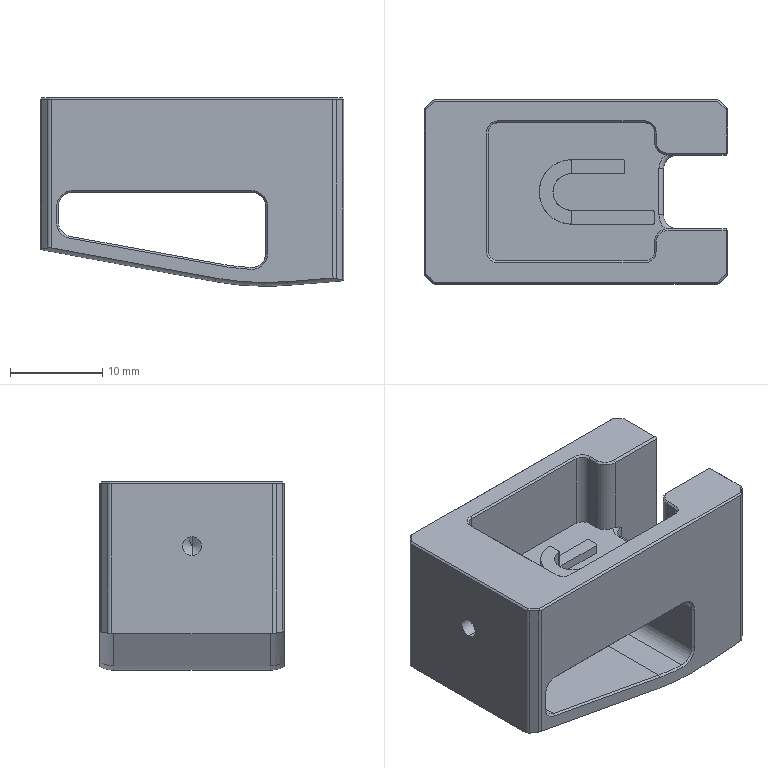NC program | NX | posted with a generic post | part box 33 x 20 x 20.478 mm
Lines 1477 to 3456 of 8500, first 1557 of 1976 lines:
(CAVITY_MILL_COPY , TOOL : D4)
N2934 T11 M6
N2936 G54
N2938 G17 G0 G90 X-6.7 Y-3.312 B0. C0. S9500 M3
N2940 G43 Z11. H11
N2942 Z1.21
N2944 G94 G1 Z-0.29 F1000.
N2946 X-7. Y-3.486
N2948 G3 X-7.5 Y-4.352 R1.
N2950 G1 Y-5.5 F1800.
N2952 X-6.352
N2954 G3 X-5.486 Y-5. R1.
N2956 G1 X-5.312 Y-4.7
N2958 Z1.21
N2960 G0 Z11.
N2962 X-6.7 Y-3.312
N2964 Z0.92
N2966 G1 Z-0.58 F1000.
N2968 X-7. Y-3.486
N2970 G3 X-7.5 Y-4.352 R1.
N2972 G1 Y-5.5 F1800.
N2974 X-6.352
N2976 G3 X-5.486 Y-5. R1.
N2978 G1 X-5.312 Y-4.7
N2980 Z0.92
N2982 G0 Z11.
N2984 X-6.7 Y-3.312
N2986 Z0.63
N2988 G1 Z-0.87 F1000.
N2990 X-7. Y-3.486
N2992 G3 X-7.5 Y-4.352 R1.
N2994 G1 Y-5.5 F1800.
N2996 X-6.352
N2998 G3 X-5.486 Y-5. R1.
N3000 G1 X-5.312 Y-4.7
N3002 Z0.63
N3004 G0 Z11.
N3006 X-6.7 Y-3.312
N3008 Z0.34
N3010 G1 Z-1.16 F1000.
N3012 X-7. Y-3.486
N3014 G3 X-7.5 Y-4.352 R1.
N3016 G1 Y-5.5 F1800.
N3018 X-6.352
N3020 G3 X-5.486 Y-5. R1.
N3022 G1 X-5.312 Y-4.7
N3024 Z0.34
N3026 G0 Z11.
N3028 X-6.7 Y-3.312
N3030 Z0.05
N3032 G1 Z-1.45 F1000.
N3034 X-7. Y-3.486
N3036 G3 X-7.5 Y-4.352 R1.
N3038 G1 Y-5.5 F1800.
N3040 X-6.352
N3042 G3 X-5.486 Y-5. R1.
N3044 G1 X-5.312 Y-4.7
N3046 Z0.05
N3048 G0 X-6.7 Y-3.312 Z-0.24
N3050 G1 Z-1.74 F1000.
N3052 X-7. Y-3.486
N3054 G3 X-7.5 Y-4.352 R1.
N3056 G1 Y-5.5 F1800.
N3058 X-6.352
N3060 G3 X-5.486 Y-5. R1.
N3062 G1 X-5.312 Y-4.7
N3064 Z-0.24
N3066 G0 X-6.7 Y-3.312 Z-0.53
N3068 G1 Z-2.03 F1000.
N3070 X-7. Y-3.486
N3072 G3 X-7.5 Y-4.352 R1.
N3074 G1 Y-5.5 F1800.
N3076 X-6.352
N3078 G3 X-5.486 Y-5. R1.
N3080 G1 X-5.312 Y-4.7
N3082 Z-0.53
N3084 G0 X-6.7 Y-3.312 Z-0.82
N3086 G1 Z-2.32 F1000.
N3088 X-7. Y-3.486
N3090 G3 X-7.5 Y-4.352 R1.
N3092 G1 Y-5.5 F1800.
N3094 X-6.352
N3096 G3 X-5.486 Y-5. R1.
N3098 G1 X-5.312 Y-4.7
N3100 Z-0.82
N3102 G0 X-6.7 Y-3.312 Z-1.11
N3104 G1 Z-2.61 F1000.
N3106 X-7. Y-3.486
N3108 G3 X-7.5 Y-4.352 R1.
N3110 G1 Y-5.5 F1800.
N3112 X-6.352
N3114 G3 X-5.486 Y-5. R1.
N3116 G1 X-5.312 Y-4.7
N3118 Z-1.11
N3120 G0 X-6.7 Y-3.312 Z-1.4
N3122 G1 Z-2.9 F1000.
N3124 X-7. Y-3.486
N3126 G3 X-7.5 Y-4.352 R1.
N3128 G1 Y-5.5 F1800.
N3130 X-6.352
N3132 G3 X-5.486 Y-5. R1.
N3134 G1 X-5.312 Y-4.7
N3136 Z-1.4
N3138 G0 X-6.7 Y-3.312 Z-1.69
N3140 G1 Z-3.19 F1000.
N3142 X-7. Y-3.486
N3144 G3 X-7.5 Y-4.352 R1.
N3146 G1 Y-5.5 F1800.
N3148 X-6.352
N3150 G3 X-5.486 Y-5. R1.
N3152 G1 X-5.312 Y-4.7
N3154 Z-1.69
N3156 G0 X-6.7 Y-3.312 Z-1.98
N3158 G1 Z-3.48 F1000.
N3160 X-7. Y-3.486
N3162 G3 X-7.5 Y-4.352 R1.
N3164 G1 Y-5.5 F1800.
N3166 X-6.352
N3168 G3 X-5.486 Y-5. R1.
N3170 G1 X-5.312 Y-4.7
N3172 Z-1.98
N3174 G0 X-6.7 Y-3.312 Z-2.27
N3176 G1 Z-3.77 F1000.
N3178 X-7. Y-3.486
N3180 G3 X-7.5 Y-4.352 R1.
N3182 G1 Y-5.5 F1800.
N3184 X-6.352
N3186 G3 X-5.486 Y-5. R1.
N3188 G1 X-5.312 Y-4.7
N3190 Z-2.27
N3192 G0 X-6.7 Y-3.312 Z-2.56
N3194 G1 Z-4.06 F1000.
N3196 X-7. Y-3.486
N3198 G3 X-7.5 Y-4.352 R1.
N3200 G1 Y-5.5 F1800.
N3202 X-6.352
N3204 G3 X-5.486 Y-5. R1.
N3206 G1 X-5.312 Y-4.7
N3208 Z-2.56
N3210 G0 X-6.7 Y-3.312 Z-2.85
N3212 G1 Z-4.35 F1000.
N3214 X-7. Y-3.486
N3216 G3 X-7.5 Y-4.352 R1.
N3218 G1 Y-5.5 F1800.
N3220 X-6.352
N3222 G3 X-5.486 Y-5. R1.
N3224 G1 X-5.312 Y-4.7
N3226 Z-2.85
N3228 G0 X-6.7 Y-3.312 Z-3.14
N3230 G1 Z-4.64 F1000.
N3232 X-7. Y-3.486
N3234 G3 X-7.5 Y-4.352 R1.
N3236 G1 Y-5.5 F1800.
N3238 X-6.352
N3240 G3 X-5.486 Y-5. R1.
N3242 G1 X-5.312 Y-4.7
N3244 Z-3.14
N3246 G0 X-6.7 Y-3.312 Z-3.43
N3248 G1 Z-4.93 F1000.
N3250 X-7. Y-3.486
N3252 G3 X-7.5 Y-4.352 R1.
N3254 G1 Y-5.5 F1800.
N3256 X-6.352
N3258 G3 X-5.486 Y-5. R1.
N3260 G1 X-5.312 Y-4.7
N3262 Z-3.43
N3264 G0 X-6.7 Y-3.312 Z-3.72
N3266 G1 Z-5.22 F1000.
N3268 X-7. Y-3.486
N3270 G3 X-7.5 Y-4.352 R1.
N3272 G1 Y-5.5 F1800.
N3274 X-6.352
N3276 G3 X-5.486 Y-5. R1.
N3278 G1 X-5.312 Y-4.7
N3280 Z-3.72
N3282 G0 X-6.7 Y-3.312 Z-4.01
N3284 G1 Z-5.51 F1000.
N3286 X-7. Y-3.486
N3288 G3 X-7.5 Y-4.352 R1.
N3290 G1 Y-5.5 F1800.
N3292 X-6.352
N3294 G3 X-5.486 Y-5. R1.
N3296 G1 X-5.312 Y-4.7
N3298 Z-4.01
N3300 G0 X-6.7 Y-3.312 Z-4.3
N3302 G1 Z-5.8 F1000.
N3304 X-7. Y-3.486
N3306 G3 X-7.5 Y-4.352 R1.
N3308 G1 Y-5.5 F1800.
N3310 X-6.352
N3312 G3 X-5.486 Y-5. R1.
N3314 G1 X-5.312 Y-4.7
N3316 Z-4.3
N3318 G0 X-6.7 Y-3.312 Z-4.586
N3320 G1 Z-6.086 F1000.
N3322 X-7. Y-3.486
N3324 G3 X-7.5 Y-4.352 R1.
N3326 G1 Y-5.5 F1800.
N3328 X-6.352
N3330 G3 X-5.486 Y-5. R1.
N3332 G1 X-5.845 Y-4.677
N3334 Z-4.586
N3336 G0 X-6.7 Y-3.312 Z-4.871
N3338 G1 Z-6.371 F1000.
N3340 X-7. Y-3.486
N3342 G3 X-7.5 Y-4.352 R1.
N3344 G1 Y-5.5 F1800.
N3346 X-6.352
N3348 G3 X-5.486 Y-5. R1.
N3350 G1 X-5.845 Y-4.677
N3352 Z-4.871
N3354 G0 X-6.7 Y-3.312 Z-5.157
N3356 G1 Z-6.657 F1000.
N3358 X-7. Y-3.486
N3360 G3 X-7.5 Y-4.352 R1.
N3362 G1 Y-5.5 F1800.
N3364 X-6.352
N3366 G3 X-5.486 Y-5. R1.
N3368 G1 X-5.845 Y-4.677
N3370 Z-5.157
N3372 G0 X-6.7 Y-3.312 Z-5.443
N3374 G1 Z-6.943 F1000.
N3376 X-7. Y-3.486
N3378 G3 X-7.5 Y-4.352 R1.
N3380 G1 Y-5.5 F1800.
N3382 X-6.352
N3384 G3 X-5.486 Y-5. R1.
N3386 G1 X-5.845 Y-4.677
N3388 Z-5.443
N3390 G0 X-6.7 Y-3.312 Z-5.729
N3392 G1 Z-7.229 F1000.
N3394 X-7. Y-3.486
N3396 G3 X-7.5 Y-4.352 R1.
N3398 G1 Y-5.5 F1800.
N3400 X-6.352
N3402 G3 X-5.486 Y-5. R1.
N3404 G1 X-5.845 Y-4.677
N3406 Z-5.729
N3408 G0 X-6.7 Y-3.312 Z-6.014
N3410 G1 Z-7.514 F1000.
N3412 X-7. Y-3.486
N3414 G3 X-7.5 Y-4.352 R1.
N3416 G1 Y-5.5 F1800.
N3418 X-6.352
N3420 G3 X-5.486 Y-5. R1.
N3422 G1 X-5.845 Y-4.677
N3424 Z-6.014
N3426 G0 X-6.7 Y-3.312 Z-6.3
N3428 G1 Z-7.8 F1000.
N3430 X-7. Y-3.486
N3432 G3 X-7.5 Y-4.352 R1.
N3434 G1 Y-5.5 F1800.
N3436 X-6.352
N3438 G3 X-5.486 Y-5. R1.
N3440 G1 X-5.845 Y-4.677
N3442 Z-6.3
N3444 G0 X-6.7 Y-3.312 Z-6.55
N3446 G1 Z-8.05 F1000.
N3448 X-7. Y-3.486
N3450 G3 X-7.5 Y-4.352 R1.
N3452 G1 Y-5.5 F1800.
N3454 X-6.352
N3456 G3 X-5.486 Y-5. R1.
N3458 G1 X-5.845 Y-4.677
N3460 Z-6.55
N3462 G0 X-6.7 Y-3.312 Z-6.8
N3464 G1 Z-8.3 F1000.
N3466 X-7. Y-3.486
N3468 G3 X-7.5 Y-4.352 R1.
N3470 G1 Y-5.5 F1800.
N3472 X-6.352
N3474 G3 X-5.486 Y-5. R1.
N3476 G1 X-5.845 Y-4.677
N3478 Z-6.8
N3480 G0 X-6.7 Y-3.312 Z-7.05
N3482 G1 Z-8.55 F1000.
N3484 X-7. Y-3.486
N3486 G3 X-7.5 Y-4.352 R1.
N3488 G1 Y-5.5 F1800.
N3490 X-6.352
N3492 G3 X-5.486 Y-5. R1.
N3494 G1 X-5.845 Y-4.677
N3496 Z-7.05
N3498 G0 X-6.7 Y-3.312 Z-7.3
N3500 G1 Z-8.8 F1000.
N3502 X-7. Y-3.486
N3504 G3 X-7.5 Y-4.352 R1.
N3506 G1 Y-5.5 F1800.
N3508 X-6.352
N3510 G3 X-5.486 Y-5. R1.
N3512 G1 X-5.845 Y-4.677
N3514 Z-7.3
N3516 G0 Z11.
N3518 X-5.518 Y-3.809
N3520 Z-4.586
N3522 G1 Z-6.086 F1000.
N3524 X-4.806 Y-3.721
N3526 G2 X-4.672 Y-4.712 R1.
N3528 X-5.005 Y-5.028 R0.56 F1800.
N3530 G3 X-5.339 Y-5.5 R0.5
N3532 G1 X2.412
N3534 G3 X2.078 Y-5.028 R0.5
N3536 G2 X1.707 Y-4.439 R0.56
N3538 G3 X1.407 Y-3.926 R0.5
N3540 G2 X-0.833 Y-5.49 R2.2
N3542 X-4.589 Y-3.678 R5.5
N3544 G3 X-4.687 Y-4.254 R0.5
N3546 G2 X-4.672 Y-4.712 R0.56
N3548 X-5.463 Y-5.324 R1.
N3550 G1 X-5.845 Y-4.677
N3552 Z-4.586
N3554 G0 X-5.518 Y-3.809 Z-4.871
N3556 G1 Z-6.371 F1000.
N3558 X-4.806 Y-3.721
N3560 G2 X-4.672 Y-4.712 R1.
N3562 X-5.005 Y-5.028 R0.56 F1800.
N3564 G3 X-5.339 Y-5.5 R0.5
N3566 G1 X2.412
N3568 G3 X2.078 Y-5.028 R0.5
N3570 G2 X1.707 Y-4.439 R0.56
N3572 G3 X1.407 Y-3.926 R0.5
N3574 G2 X-0.833 Y-5.49 R2.2
N3576 X-4.589 Y-3.678 R5.5
N3578 G3 X-4.687 Y-4.254 R0.5
N3580 G2 X-4.672 Y-4.712 R0.56
N3582 X-5.463 Y-5.324 R1.
N3584 G1 X-5.845 Y-4.677
N3586 Z-4.871
N3588 G0 X-5.518 Y-3.809 Z-5.157
N3590 G1 Z-6.657 F1000.
N3592 X-4.806 Y-3.721
N3594 G2 X-4.672 Y-4.712 R1.
N3596 X-5.005 Y-5.028 R0.56 F1800.
N3598 G3 X-5.339 Y-5.5 R0.5
N3600 G1 X2.412
N3602 G3 X2.078 Y-5.028 R0.5
N3604 G2 X1.707 Y-4.439 R0.56
N3606 G3 X1.407 Y-3.926 R0.5
N3608 G2 X-0.833 Y-5.49 R2.2
N3610 X-4.589 Y-3.678 R5.5
N3612 G3 X-4.687 Y-4.254 R0.5
N3614 G2 X-4.672 Y-4.712 R0.56
N3616 X-5.463 Y-5.324 R1.
N3618 G1 X-5.845 Y-4.677
N3620 Z-5.157
N3622 G0 X-5.518 Y-3.809 Z-5.443
N3624 G1 Z-6.943 F1000.
N3626 X-4.806 Y-3.721
N3628 G2 X-4.672 Y-4.712 R1.
N3630 X-5.005 Y-5.028 R0.56 F1800.
N3632 G3 X-5.339 Y-5.5 R0.5
N3634 G1 X2.412
N3636 G3 X2.078 Y-5.028 R0.5
N3638 G2 X1.707 Y-4.439 R0.56
N3640 G3 X1.407 Y-3.926 R0.5
N3642 G2 X-0.833 Y-5.49 R2.2
N3644 X-4.589 Y-3.678 R5.5
N3646 G3 X-4.687 Y-4.254 R0.5
N3648 G2 X-4.672 Y-4.712 R0.56
N3650 X-5.463 Y-5.324 R1.
N3652 G1 X-5.845 Y-4.677
N3654 Z-5.443
N3656 G0 X-5.518 Y-3.809 Z-5.729
N3658 G1 Z-7.229 F1000.
N3660 X-4.806 Y-3.721
N3662 G2 X-4.672 Y-4.712 R1.
N3664 X-5.005 Y-5.028 R0.56 F1800.
N3666 G3 X-5.339 Y-5.5 R0.5
N3668 G1 X2.412
N3670 G3 X2.078 Y-5.028 R0.5
N3672 G2 X1.707 Y-4.439 R0.56
N3674 G3 X1.407 Y-3.926 R0.5
N3676 G2 X-0.833 Y-5.49 R2.2
N3678 X-4.589 Y-3.678 R5.5
N3680 G3 X-4.687 Y-4.254 R0.5
N3682 G2 X-4.672 Y-4.712 R0.56
N3684 X-5.463 Y-5.324 R1.
N3686 G1 X-5.845 Y-4.677
N3688 Z-5.729
N3690 G0 X-5.518 Y-3.809 Z-6.014
N3692 G1 Z-7.514 F1000.
N3694 X-4.806 Y-3.721
N3696 G2 X-4.672 Y-4.712 R1.
N3698 X-5.005 Y-5.028 R0.56 F1800.
N3700 G3 X-5.339 Y-5.5 R0.5
N3702 G1 X2.412
N3704 G3 X2.078 Y-5.028 R0.5
N3706 G2 X1.707 Y-4.439 R0.56
N3708 G3 X1.407 Y-3.926 R0.5
N3710 G2 X-0.833 Y-5.49 R2.2
N3712 X-4.589 Y-3.678 R5.5
N3714 G3 X-4.687 Y-4.254 R0.5
N3716 G2 X-4.672 Y-4.712 R0.56
N3718 X-5.463 Y-5.324 R1.
N3720 G1 X-5.845 Y-4.677
N3722 Z-6.014
N3724 G0 X-5.518 Y-3.809 Z-6.3
N3726 G1 Z-7.8 F1000.
N3728 X-4.806 Y-3.721
N3730 G2 X-4.672 Y-4.712 R1.
N3732 X-5.005 Y-5.028 R0.56 F1800.
N3734 G3 X-5.339 Y-5.5 R0.5
N3736 G1 X2.412
N3738 G3 X2.078 Y-5.028 R0.5
N3740 G2 X1.707 Y-4.439 R0.56
N3742 G3 X1.407 Y-3.926 R0.5
N3744 G2 X-0.833 Y-5.49 R2.2
N3746 X-4.589 Y-3.678 R5.5
N3748 G3 X-4.687 Y-4.254 R0.5
N3750 G2 X-4.672 Y-4.712 R0.56
N3752 X-5.463 Y-5.324 R1.
N3754 G1 X-5.845 Y-4.677
N3756 Z-6.3
N3758 G0 Z-6.55
N3760 G1 Z-8.05 F1000.
N3762 X-6.205 Y-5.
N3764 G3 X-5.339 Y-5.5 R1.
N3766 G1 X-0.5 F1800.
N3768 G2 X-4.589 Y-3.678 R5.5
N3770 G3 X-5.54 Y-3.369 R1.
N3772 G1 X-5.79 Y-3.422
N3774 Z-6.55
N3776 G0 X-5.845 Y-4.677 Z-6.8
N3778 G1 Z-8.3 F1000.
N3780 X-6.205 Y-5.
N3782 G3 X-5.339 Y-5.5 R1.
N3784 G1 X-0.5 F1800.
N3786 G2 X-4.589 Y-3.678 R5.5
N3788 G3 X-5.54 Y-3.369 R1.
N3790 G1 X-5.79 Y-3.422
N3792 Z-6.8
N3794 G0 X-5.845 Y-4.677 Z-7.05
N3796 G1 Z-8.55 F1000.
N3798 X-6.205 Y-5.
N3800 G3 X-5.339 Y-5.5 R1.
N3802 G1 X-0.5 F1800.
N3804 G2 X-4.589 Y-3.678 R5.5
N3806 G3 X-5.54 Y-3.369 R1.
N3808 G1 X-5.79 Y-3.422
N3810 Z-7.05
N3812 G0 X-5.845 Y-4.677 Z-7.3
N3814 G1 Z-8.8 F1000.
N3816 X-6.205 Y-5.
N3818 G3 X-5.339 Y-5.5 R1.
N3820 G1 X-0.5 F1800.
N3822 G2 X-4.589 Y-3.678 R5.5
N3824 G3 X-5.54 Y-3.369 R1.
N3826 G1 X-5.79 Y-3.422
N3828 Z-7.3
N3830 G0 Z11.
N3832 X-5.312 Y4.7
N3834 Z1.21
N3836 G1 Z-0.29 F1000.
N3838 X-5.486 Y5.
N3840 G3 X-6.352 Y5.5 R1.
N3842 G1 X-7.5 F1800.
N3844 Y4.352
N3846 G3 X-7. Y3.486 R1.
N3848 G1 X-6.7 Y3.312
N3850 Z1.21
N3852 G0 Z11.
N3854 X-5.312 Y4.7
N3856 Z0.92
N3858 G1 Z-0.58 F1000.
N3860 X-5.486 Y5.
N3862 G3 X-6.352 Y5.5 R1.
N3864 G1 X-7.5 F1800.
N3866 Y4.352
N3868 G3 X-7. Y3.486 R1.
N3870 G1 X-6.7 Y3.312
N3872 Z0.92
N3874 G0 Z11.
N3876 X-5.312 Y4.7
N3878 Z0.63
N3880 G1 Z-0.87 F1000.
N3882 X-5.486 Y5.
N3884 G3 X-6.352 Y5.5 R1.
N3886 G1 X-7.5 F1800.
N3888 Y4.352
N3890 G3 X-7. Y3.486 R1.
N3892 G1 X-6.7 Y3.312
N3894 Z0.63
N3896 G0 Z11.
N3898 X-5.312 Y4.7
N3900 Z0.34
N3902 G1 Z-1.16 F1000.
N3904 X-5.486 Y5.
N3906 G3 X-6.352 Y5.5 R1.
N3908 G1 X-7.5 F1800.
N3910 Y4.352
N3912 G3 X-7. Y3.486 R1.
N3914 G1 X-6.7 Y3.312
N3916 Z0.34
N3918 G0 Z11.
N3920 X-5.312 Y4.7
N3922 Z0.05
N3924 G1 Z-1.45 F1000.
N3926 X-5.486 Y5.
N3928 G3 X-6.352 Y5.5 R1.
N3930 G1 X-7.5 F1800.
N3932 Y4.352
N3934 G3 X-7. Y3.486 R1.
N3936 G1 X-6.7 Y3.312
N3938 Z0.05
N3940 G0 X-5.312 Y4.7 Z-0.24
N3942 G1 Z-1.74 F1000.
N3944 X-5.486 Y5.
N3946 G3 X-6.352 Y5.5 R1.
N3948 G1 X-7.5 F1800.
N3950 Y4.352
N3952 G3 X-7. Y3.486 R1.
N3954 G1 X-6.7 Y3.312
N3956 Z-0.24
N3958 G0 X-5.312 Y4.7 Z-0.53
N3960 G1 Z-2.03 F1000.
N3962 X-5.486 Y5.
N3964 G3 X-6.352 Y5.5 R1.
N3966 G1 X-7.5 F1800.
N3968 Y4.352
N3970 G3 X-7. Y3.486 R1.
N3972 G1 X-6.7 Y3.312
N3974 Z-0.53
N3976 G0 X-5.312 Y4.7 Z-0.82
N3978 G1 Z-2.32 F1000.
N3980 X-5.486 Y5.
N3982 G3 X-6.352 Y5.5 R1.
N3984 G1 X-7.5 F1800.
N3986 Y4.352
N3988 G3 X-7. Y3.486 R1.
N3990 G1 X-6.7 Y3.312
N3992 Z-0.82
N3994 G0 X-5.312 Y4.7 Z-1.11
N3996 G1 Z-2.61 F1000.
N3998 X-5.486 Y5.
N4000 G3 X-6.352 Y5.5 R1.
N4002 G1 X-7.5 F1800.
N4004 Y4.352
N4006 G3 X-7. Y3.486 R1.
N4008 G1 X-6.7 Y3.312
N4010 Z-1.11
N4012 G0 X-5.312 Y4.7 Z-1.4
N4014 G1 Z-2.9 F1000.
N4016 X-5.486 Y5.
N4018 G3 X-6.352 Y5.5 R1.
N4020 G1 X-7.5 F1800.
N4022 Y4.352
N4024 G3 X-7. Y3.486 R1.
N4026 G1 X-6.7 Y3.312
N4028 Z-1.4
N4030 G0 X-5.312 Y4.7 Z-1.69
N4032 G1 Z-3.19 F1000.
N4034 X-5.486 Y5.
N4036 G3 X-6.352 Y5.5 R1.
N4038 G1 X-7.5 F1800.
N4040 Y4.352
N4042 G3 X-7. Y3.486 R1.
N4044 G1 X-6.7 Y3.312
N4046 Z-1.69
N4048 G0 X-5.312 Y4.7 Z-1.98
N4050 G1 Z-3.48 F1000.
N4052 X-5.486 Y5.
N4054 G3 X-6.352 Y5.5 R1.
N4056 G1 X-7.5 F1800.
N4058 Y4.352
N4060 G3 X-7. Y3.486 R1.
N4062 G1 X-6.7 Y3.312
N4064 Z-1.98
N4066 G0 X-5.312 Y4.7 Z-2.27
N4068 G1 Z-3.77 F1000.
N4070 X-5.486 Y5.
N4072 G3 X-6.352 Y5.5 R1.
N4074 G1 X-7.5 F1800.
N4076 Y4.352
N4078 G3 X-7. Y3.486 R1.
N4080 G1 X-6.7 Y3.312
N4082 Z-2.27
N4084 G0 X-5.312 Y4.7 Z-2.56
N4086 G1 Z-4.06 F1000.
N4088 X-5.486 Y5.
N4090 G3 X-6.352 Y5.5 R1.
N4092 G1 X-7.5 F1800.
N4094 Y4.352
N4096 G3 X-7. Y3.486 R1.
N4098 G1 X-6.7 Y3.312
N4100 Z-2.56
N4102 G0 X-5.312 Y4.7 Z-2.85
N4104 G1 Z-4.35 F1000.
N4106 X-5.486 Y5.
N4108 G3 X-6.352 Y5.5 R1.
N4110 G1 X-7.5 F1800.
N4112 Y4.352
N4114 G3 X-7. Y3.486 R1.
N4116 G1 X-6.7 Y3.312
N4118 Z-2.85
N4120 G0 X-5.312 Y4.7 Z-3.14
N4122 G1 Z-4.64 F1000.
N4124 X-5.486 Y5.
N4126 G3 X-6.352 Y5.5 R1.
N4128 G1 X-7.5 F1800.
N4130 Y4.352
N4132 G3 X-7. Y3.486 R1.
N4134 G1 X-6.7 Y3.312
N4136 Z-3.14
N4138 G0 X-5.312 Y4.7 Z-3.43
N4140 G1 Z-4.93 F1000.
N4142 X-5.486 Y5.
N4144 G3 X-6.352 Y5.5 R1.
N4146 G1 X-7.5 F1800.
N4148 Y4.352
N4150 G3 X-7. Y3.486 R1.
N4152 G1 X-6.7 Y3.312
N4154 Z-3.43
N4156 G0 X-5.312 Y4.7 Z-3.72
N4158 G1 Z-5.22 F1000.
N4160 X-5.486 Y5.
N4162 G3 X-6.352 Y5.5 R1.
N4164 G1 X-7.5 F1800.
N4166 Y4.352
N4168 G3 X-7. Y3.486 R1.
N4170 G1 X-6.7 Y3.312
N4172 Z-3.72
N4174 G0 X-5.312 Y4.7 Z-4.01
N4176 G1 Z-5.51 F1000.
N4178 X-5.486 Y5.
N4180 G3 X-6.352 Y5.5 R1.
N4182 G1 X-7.5 F1800.
N4184 Y4.352
N4186 G3 X-7. Y3.486 R1.
N4188 G1 X-6.7 Y3.312
N4190 Z-4.01
N4192 G0 X-5.312 Y4.7 Z-4.3
N4194 G1 Z-5.8 F1000.
N4196 X-5.486 Y5.
N4198 G3 X-6.352 Y5.5 R1.
N4200 G1 X-7.5 F1800.
N4202 Y4.352
N4204 G3 X-7. Y3.486 R1.
N4206 G1 X-6.7 Y3.312
N4208 Z-4.3
N4210 G0 X-6.429 Y-2.885 Z-4.586
N4212 G1 Z-6.086 F1000.
N4214 X-6.773 Y-2.576
N4216 G2 X-5.812 Y-2.299 R1.
N4218 G3 X-5.506 Y-2.277 R0.5 F1800.
N4220 G2 X-5.506 Y2.277 R5.5
N4222 G3 X-6.073 Y2.137 R0.5
N4224 G1 X-6.177 Y2.042
N4226 G3 X-6.5 Y1.771 R2.5
N4228 X-6.823 Y2.042 R2.5
N4230 G2 X-7.028 Y2.314 R0.56
N4232 G3 X-7.5 Y2.648 R0.5
N4234 G1 Y-2.648
N4236 G3 X-7.028 Y-2.314 R0.5
N4238 G2 X-6.823 Y-2.042 R0.56
N4240 G3 X-6.5 Y-1.771 R2.5
N4242 X-6.177 Y-2.042 R2.5
N4244 G1 X-6.073 Y-2.137
N4246 G3 X-5.812 Y-2.299 R0.5
N4248 G2 X-5.452 Y-2.645 R0.5
N4250 G1 X-5.997 Y-3.077
N4252 Z-4.586
N4254 G0 X-6.429 Y-2.885 Z-4.871
N4256 G1 Z-6.371 F1000.
N4258 X-6.773 Y-2.576
N4260 G2 X-5.812 Y-2.299 R1.
N4262 G3 X-5.506 Y-2.277 R0.5 F1800.
N4264 G2 X-5.506 Y2.277 R5.5
N4266 G3 X-6.073 Y2.137 R0.5
N4268 G1 X-6.177 Y2.042
N4270 G3 X-6.5 Y1.771 R2.5
N4272 X-6.823 Y2.042 R2.5
N4274 G2 X-7.028 Y2.314 R0.56
N4276 G3 X-7.5 Y2.648 R0.5
N4278 G1 Y-2.648
N4280 G3 X-7.028 Y-2.314 R0.5
N4282 G2 X-6.823 Y-2.042 R0.56
N4284 G3 X-6.5 Y-1.771 R2.5
N4286 X-6.177 Y-2.042 R2.5
N4288 G1 X-6.073 Y-2.137
N4290 G3 X-5.812 Y-2.299 R0.5
N4292 G2 X-5.452 Y-2.645 R0.5
N4294 G1 X-5.997 Y-3.077
N4296 Z-4.871
N4298 G0 X-6.429 Y-2.885 Z-5.157
N4300 G1 Z-6.657 F1000.
N4302 X-6.773 Y-2.576
N4304 G2 X-5.812 Y-2.299 R1.
N4306 G3 X-5.506 Y-2.277 R0.5 F1800.
N4308 G2 X-5.506 Y2.277 R5.5
N4310 G3 X-6.073 Y2.137 R0.5
N4312 G1 X-6.177 Y2.042
N4314 G3 X-6.5 Y1.771 R2.5
N4316 X-6.823 Y2.042 R2.5
N4318 G2 X-7.028 Y2.314 R0.56
N4320 G3 X-7.5 Y2.648 R0.5
N4322 G1 Y-2.648
N4324 G3 X-7.028 Y-2.314 R0.5
N4326 G2 X-6.823 Y-2.042 R0.56
N4328 G3 X-6.5 Y-1.771 R2.5
N4330 X-6.177 Y-2.042 R2.5
N4332 G1 X-6.073 Y-2.137
N4334 G3 X-5.812 Y-2.299 R0.5
N4336 G2 X-5.452 Y-2.645 R0.5
N4338 G1 X-5.997 Y-3.077
N4340 Z-5.157
N4342 G0 X-6.429 Y-2.885 Z-5.443
N4344 G1 Z-6.943 F1000.
N4346 X-6.773 Y-2.576
N4348 G2 X-5.812 Y-2.299 R1.
N4350 G3 X-5.506 Y-2.277 R0.5 F1800.
N4352 G2 X-5.506 Y2.277 R5.5
N4354 G3 X-6.073 Y2.137 R0.5
N4356 G1 X-6.177 Y2.042
N4358 G3 X-6.5 Y1.771 R2.5
N4360 X-6.823 Y2.042 R2.5
N4362 G2 X-7.028 Y2.314 R0.56
N4364 G3 X-7.5 Y2.648 R0.5
N4366 G1 Y-2.648
N4368 G3 X-7.028 Y-2.314 R0.5
N4370 G2 X-6.823 Y-2.042 R0.56
N4372 G3 X-6.5 Y-1.771 R2.5
N4374 X-6.177 Y-2.042 R2.5
N4376 G1 X-6.073 Y-2.137
N4378 G3 X-5.812 Y-2.299 R0.5
N4380 G2 X-5.452 Y-2.645 R0.5
N4382 G1 X-5.997 Y-3.077
N4384 Z-5.443
N4386 G0 X-6.429 Y-2.885 Z-5.729
N4388 G1 Z-7.229 F1000.
N4390 X-6.773 Y-2.576
N4392 G2 X-5.812 Y-2.299 R1.
N4394 G3 X-5.506 Y-2.277 R0.5 F1800.
N4396 G2 X-5.506 Y2.277 R5.5
N4398 G3 X-6.073 Y2.137 R0.5
N4400 G1 X-6.177 Y2.042
N4402 G3 X-6.5 Y1.771 R2.5
N4404 X-6.823 Y2.042 R2.5
N4406 G2 X-7.028 Y2.314 R0.56
N4408 G3 X-7.5 Y2.648 R0.5
N4410 G1 Y-2.648
N4412 G3 X-7.028 Y-2.314 R0.5
N4414 G2 X-6.823 Y-2.042 R0.56
N4416 G3 X-6.5 Y-1.771 R2.5
N4418 X-6.177 Y-2.042 R2.5
N4420 G1 X-6.073 Y-2.137
N4422 G3 X-5.812 Y-2.299 R0.5
N4424 G2 X-5.452 Y-2.645 R0.5
N4426 G1 X-5.997 Y-3.077
N4428 Z-5.729
N4430 G0 X-6.429 Y-2.885 Z-6.014
N4432 G1 Z-7.514 F1000.
N4434 X-6.773 Y-2.576
N4436 G2 X-5.812 Y-2.299 R1.
N4438 G3 X-5.506 Y-2.277 R0.5 F1800.
N4440 G2 X-5.506 Y2.277 R5.5
N4442 G3 X-6.073 Y2.137 R0.5
N4444 G1 X-6.177 Y2.042
N4446 G3 X-6.5 Y1.771 R2.5
N4448 X-6.823 Y2.042 R2.5
N4450 G2 X-7.028 Y2.314 R0.56
N4452 G3 X-7.5 Y2.648 R0.5
N4454 G1 Y-2.648
N4456 G3 X-7.028 Y-2.314 R0.5
N4458 G2 X-6.823 Y-2.042 R0.56
N4460 G3 X-6.5 Y-1.771 R2.5
N4462 X-6.177 Y-2.042 R2.5
N4464 G1 X-6.073 Y-2.137
N4466 G3 X-5.812 Y-2.299 R0.5
N4468 G2 X-5.452 Y-2.645 R0.5
N4470 G1 X-5.997 Y-3.077
N4472 Z-6.014
N4474 G0 X-6.429 Y-2.885 Z-6.3
N4476 G1 Z-7.8 F1000.
N4478 X-6.773 Y-2.576
N4480 G2 X-5.812 Y-2.299 R1.
N4482 G3 X-5.506 Y-2.277 R0.5 F1800.
N4484 G2 X-5.506 Y2.277 R5.5
N4486 G3 X-6.073 Y2.137 R0.5
N4488 G1 X-6.177 Y2.042
N4490 G3 X-6.5 Y1.771 R2.5
N4492 X-6.823 Y2.042 R2.5
N4494 G2 X-7.028 Y2.314 R0.56
N4496 G3 X-7.5 Y2.648 R0.5
N4498 G1 Y-2.648
N4500 G3 X-7.028 Y-2.314 R0.5
N4502 G2 X-6.823 Y-2.042 R0.56
N4504 G3 X-6.5 Y-1.771 R2.5
N4506 X-6.177 Y-2.042 R2.5
N4508 G1 X-6.073 Y-2.137
N4510 G3 X-5.812 Y-2.299 R0.5
N4512 G2 X-5.452 Y-2.645 R0.5
N4514 G1 X-5.997 Y-3.077
N4516 Z-6.3
N4518 G0 X-6.429 Y-2.885 Z-6.55
N4520 G1 Z-8.05 F1000.
N4522 X-6.773 Y-2.576
N4524 G2 X-5.812 Y-2.299 R1.
N4526 G3 X-5.506 Y-2.277 R0.5 F1800.
N4528 G2 X-5.506 Y2.277 R5.5
N4530 G3 X-6.073 Y2.137 R0.5
N4532 G1 X-6.177 Y2.042
N4534 G3 X-6.5 Y1.771 R2.5
N4536 X-6.823 Y2.042 R2.5
N4538 G2 X-7.028 Y2.314 R0.56
N4540 G3 X-7.5 Y2.648 R0.5
N4542 G1 Y-2.648
N4544 G3 X-7.028 Y-2.314 R0.5
N4546 G2 X-6.823 Y-2.042 R0.56
N4548 G3 X-6.5 Y-1.771 R2.5
N4550 X-6.177 Y-2.042 R2.5
N4552 G1 X-6.073 Y-2.137
N4554 G3 X-5.812 Y-2.299 R0.5
N4556 G2 X-5.452 Y-2.645 R0.5
N4558 G1 X-5.997 Y-3.077
N4560 Z-6.55
N4562 G0 X-6.429 Y-2.885 Z-6.8
N4564 G1 Z-8.3 F1000.
N4566 X-6.773 Y-2.576
N4568 G2 X-5.812 Y-2.299 R1.
N4570 G3 X-5.506 Y-2.277 R0.5 F1800.
N4572 G2 X-5.506 Y2.277 R5.5
N4574 G3 X-6.073 Y2.137 R0.5
N4576 G1 X-6.177 Y2.042
N4578 G3 X-6.5 Y1.771 R2.5
N4580 X-6.823 Y2.042 R2.5
N4582 G2 X-7.028 Y2.314 R0.56
N4584 G3 X-7.5 Y2.648 R0.5
N4586 G1 Y-2.648
N4588 G3 X-7.028 Y-2.314 R0.5
N4590 G2 X-6.823 Y-2.042 R0.56
N4592 G3 X-6.5 Y-1.771 R2.5
N4594 X-6.177 Y-2.042 R2.5
N4596 G1 X-6.073 Y-2.137
N4598 G3 X-5.812 Y-2.299 R0.5
N4600 G2 X-5.452 Y-2.645 R0.5
N4602 G1 X-5.997 Y-3.077
N4604 Z-6.8
N4606 G0 X-6.429 Y-2.885 Z-7.05
N4608 G1 Z-8.55 F1000.
N4610 X-6.773 Y-2.576
N4612 G2 X-5.812 Y-2.299 R1.
N4614 G3 X-5.506 Y-2.277 R0.5 F1800.
N4616 G2 X-5.506 Y2.277 R5.5
N4618 G3 X-6.073 Y2.137 R0.5
N4620 G1 X-6.177 Y2.042
N4622 G3 X-6.5 Y1.771 R2.5
N4624 X-6.823 Y2.042 R2.5
N4626 G2 X-7.028 Y2.314 R0.56
N4628 G3 X-7.5 Y2.648 R0.5
N4630 G1 Y-2.648
N4632 G3 X-7.028 Y-2.314 R0.5
N4634 G2 X-6.823 Y-2.042 R0.56
N4636 G3 X-6.5 Y-1.771 R2.5
N4638 X-6.177 Y-2.042 R2.5
N4640 G1 X-6.073 Y-2.137
N4642 G3 X-5.812 Y-2.299 R0.5
N4644 G2 X-5.452 Y-2.645 R0.5
N4646 G1 X-5.997 Y-3.077
N4648 Z-7.05
N4650 G0 X-6.429 Y-2.885 Z-7.3
N4652 G1 Z-8.8 F1000.
N4654 X-6.773 Y-2.576
N4656 G2 X-5.812 Y-2.299 R1.
N4658 G3 X-5.506 Y-2.277 R0.5 F1800.
N4660 G2 X-5.506 Y2.277 R5.5
N4662 G3 X-6.073 Y2.137 R0.5
N4664 G1 X-6.177 Y2.042
N4666 G3 X-6.5 Y1.771 R2.5
N4668 X-6.823 Y2.042 R2.5
N4670 G2 X-7.028 Y2.314 R0.56
N4672 G3 X-7.5 Y2.648 R0.5
N4674 G1 Y-2.648
N4676 G3 X-7.028 Y-2.314 R0.5
N4678 G2 X-6.823 Y-2.042 R0.56
N4680 G3 X-6.5 Y-1.771 R2.5
N4682 X-6.177 Y-2.042 R2.5
N4684 G1 X-6.073 Y-2.137
N4686 G3 X-5.812 Y-2.299 R0.5
N4688 G2 X-5.452 Y-2.645 R0.5
N4690 G1 X-5.997 Y-3.077
N4692 Z-7.3
N4694 G0 Z11.
N4696 X-5.864 Y4.655
N4698 Z-4.586
N4700 G1 Z-6.086 F1000.
N4702 X-5.486 Y5.
N4704 G3 X-6.352 Y5.5 R1.
N4706 G1 X-7.5 F1800.
N4708 Y4.352
N4710 G3 X-7. Y3.486 R1.
N4712 G1 X-6.7 Y3.312
N4714 Z-4.586
N4716 G0 X-5.864 Y4.655 Z-4.871
N4718 G1 Z-6.371 F1000.
N4720 X-5.486 Y5.
N4722 G3 X-6.352 Y5.5 R1.
N4724 G1 X-7.5 F1800.
N4726 Y4.352
N4728 G3 X-7. Y3.486 R1.
N4730 G1 X-6.7 Y3.312
N4732 Z-4.871
N4734 G0 X-5.864 Y4.655 Z-5.157
N4736 G1 Z-6.657 F1000.
N4738 X-5.486 Y5.
N4740 G3 X-6.352 Y5.5 R1.
N4742 G1 X-7.5 F1800.
N4744 Y4.352
N4746 G3 X-7. Y3.486 R1.
N4748 G1 X-6.7 Y3.312
N4750 Z-5.157
N4752 G0 X-5.864 Y4.655 Z-5.443
N4754 G1 Z-6.943 F1000.
N4756 X-5.486 Y5.
N4758 G3 X-6.352 Y5.5 R1.
N4760 G1 X-7.5 F1800.
N4762 Y4.352
N4764 G3 X-7. Y3.486 R1.
N4766 G1 X-6.7 Y3.312
N4768 Z-5.443
N4770 G0 X-5.864 Y4.655 Z-5.729
N4772 G1 Z-7.229 F1000.
N4774 X-5.486 Y5.
N4776 G3 X-6.352 Y5.5 R1.
N4778 G1 X-7.5 F1800.
N4780 Y4.352
N4782 G3 X-7. Y3.486 R1.
N4784 G1 X-6.7 Y3.312
N4786 Z-5.729
N4788 G0 X-5.864 Y4.655 Z-6.014
N4790 G1 Z-7.514 F1000.
N4792 X-5.486 Y5.
N4794 G3 X-6.352 Y5.5 R1.
N4796 G1 X-7.5 F1800.
N4798 Y4.352
N4800 G3 X-7. Y3.486 R1.
N4802 G1 X-6.7 Y3.312
N4804 Z-6.014
N4806 G0 X-5.864 Y4.655 Z-6.3
N4808 G1 Z-7.8 F1000.
N4810 X-5.486 Y5.
N4812 G3 X-6.352 Y5.5 R1.
N4814 G1 X-7.5 F1800.
N4816 Y4.352
N4818 G3 X-7. Y3.486 R1.
N4820 G1 X-6.7 Y3.312
N4822 Z-6.3
N4824 G0 X-5.864 Y4.655 Z-6.55
N4826 G1 Z-8.05 F1000.
N4828 X-5.486 Y5.
N4830 G3 X-6.352 Y5.5 R1.
N4832 G1 X-7.5 F1800.
N4834 Y4.352
N4836 G3 X-7. Y3.486 R1.
N4838 G1 X-6.7 Y3.312
N4840 Z-6.55
N4842 G0 X-5.864 Y4.655 Z-6.8
N4844 G1 Z-8.3 F1000.
N4846 X-5.486 Y5.
N4848 G3 X-6.352 Y5.5 R1.
N4850 G1 X-7.5 F1800.
N4852 Y4.352
N4854 G3 X-7. Y3.486 R1.
N4856 G1 X-6.7 Y3.312
N4858 Z-6.8
N4860 G0 X-5.864 Y4.655 Z-7.05
N4862 G1 Z-8.55 F1000.
N4864 X-5.486 Y5.
N4866 G3 X-6.352 Y5.5 R1.
N4868 G1 X-7.5 F1800.
N4870 Y4.352
N4872 G3 X-7. Y3.486 R1.
N4874 G1 X-6.7 Y3.312
N4876 Z-7.05
N4878 G0 X-5.864 Y4.655 Z-7.3
N4880 G1 Z-8.8 F1000.
N4882 X-5.486 Y5.
N4884 G3 X-6.352 Y5.5 R1.
N4886 G1 X-7.5 F1800.
N4888 Y4.352
N4890 G3 X-7. Y3.486 R1.
N4892 G1 X-6.7 Y3.312
N4894 Z-7.3
N4896 G0 Z11.
N4898 X-5.864 Y4.655
N4900 Z-4.586
N4902 G1 Z-6.086 F1000.
N4904 X-5.469 Y5.334
N4906 G2 X-4.702 Y4.692 R1.
N4908 X-4.745 Y4.216 R0.56 F1800.
N4910 G3 X-4.658 Y3.6 R0.5
N4912 G2 X-0.833 Y5.49 R5.5
N4914 X1.407 Y3.926 R2.2
N4916 G3 X1.707 Y4.439 R0.5
N4918 G2 X2.078 Y5.028 R0.56
N4920 G3 X2.412 Y5.5 R0.5
N4922 G1 X-5.376
N4924 G3 X-5.042 Y5.028 R0.5
N4926 G2 X-4.702 Y4.692 R0.56
N4928 X-4.874 Y3.707 R1.
N4930 G1 X-5.589 Y3.713
N4932 Z-4.586
N4934 G0 X-5.864 Y4.655 Z-4.871
N4936 G1 Z-6.371 F1000.
N4938 X-5.469 Y5.334
N4940 G2 X-4.702 Y4.692 R1.
N4942 X-4.745 Y4.216 R0.56 F1800.
N4944 G3 X-4.658 Y3.6 R0.5
N4946 G2 X-0.833 Y5.49 R5.5
N4948 X1.407 Y3.926 R2.2
N4950 G3 X1.707 Y4.439 R0.5
N4952 G2 X2.078 Y5.028 R0.56
N4954 G3 X2.412 Y5.5 R0.5
N4956 G1 X-5.376
N4958 G3 X-5.042 Y5.028 R0.5
N4960 G2 X-4.702 Y4.692 R0.56
N4962 X-4.874 Y3.707 R1.
N4964 G1 X-5.589 Y3.713
N4966 Z-4.871
N4968 G0 X-5.864 Y4.655 Z-5.157
N4970 G1 Z-6.657 F1000.
N4972 X-5.469 Y5.334
N4974 G2 X-4.702 Y4.692 R1.
N4976 X-4.745 Y4.216 R0.56 F1800.
N4978 G3 X-4.658 Y3.6 R0.5
N4980 G2 X-0.833 Y5.49 R5.5
N4982 X1.407 Y3.926 R2.2
N4984 G3 X1.707 Y4.439 R0.5
N4986 G2 X2.078 Y5.028 R0.56
N4988 G3 X2.412 Y5.5 R0.5
N4990 G1 X-5.376
N4992 G3 X-5.042 Y5.028 R0.5
N4994 G2 X-4.702 Y4.692 R0.56
N4996 X-4.874 Y3.707 R1.
N4998 G1 X-5.589 Y3.713
N5000 Z-5.157
N5002 G0 X-5.864 Y4.655 Z-5.443
N5004 G1 Z-6.943 F1000.
N5006 X-5.469 Y5.334
N5008 G2 X-4.702 Y4.692 R1.
N5010 X-4.745 Y4.216 R0.56 F1800.
N5012 G3 X-4.658 Y3.6 R0.5
N5014 G2 X-0.833 Y5.49 R5.5
N5016 X1.407 Y3.926 R2.2
N5018 G3 X1.707 Y4.439 R0.5
N5020 G2 X2.078 Y5.028 R0.56
N5022 G3 X2.412 Y5.5 R0.5
N5024 G1 X-5.376
N5026 G3 X-5.042 Y5.028 R0.5
N5028 G2 X-4.702 Y4.692 R0.56
N5030 X-4.874 Y3.707 R1.
N5032 G1 X-5.589 Y3.713
N5034 Z-5.443
N5036 G0 X-5.864 Y4.655 Z-5.729
N5038 G1 Z-7.229 F1000.
N5040 X-5.469 Y5.334
N5042 G2 X-4.702 Y4.692 R1.
N5044 X-4.745 Y4.216 R0.56 F1800.
N5046 G3 X-4.658 Y3.6 R0.5
N5048 G2 X-0.833 Y5.49 R5.5
N5050 X1.407 Y3.926 R2.2
N5052 G3 X1.707 Y4.439 R0.5
N5054 G2 X2.078 Y5.028 R0.56
N5056 G3 X2.412 Y5.5 R0.5
N5058 G1 X-5.376
N5060 G3 X-5.042 Y5.028 R0.5
N5062 G2 X-4.702 Y4.692 R0.56
N5064 X-4.874 Y3.707 R1.
N5066 G1 X-5.589 Y3.713
N5068 Z-5.729
N5070 G0 X-5.864 Y4.655 Z-6.014
N5072 G1 Z-7.514 F1000.
N5074 X-5.469 Y5.334
N5076 G2 X-4.702 Y4.692 R1.
N5078 X-4.745 Y4.216 R0.56 F1800.
N5080 G3 X-4.658 Y3.6 R0.5
N5082 G2 X-0.833 Y5.49 R5.5
N5084 X1.407 Y3.926 R2.2
N5086 G3 X1.707 Y4.439 R0.5
N5088 G2 X2.078 Y5.028 R0.56
N5090 G3 X2.412 Y5.5 R0.5
N5092 G1 X-5.376
N5094 G3 X-5.042 Y5.028 R0.5
N5096 G2 X-4.702 Y4.692 R0.56
N5098 X-4.874 Y3.707 R1.
N5100 G1 X-5.589 Y3.713
N5102 Z-6.014
N5104 G0 X-5.864 Y4.655 Z-6.3
N5106 G1 Z-7.8 F1000.
N5108 X-5.469 Y5.334
N5110 G2 X-4.702 Y4.692 R1.
N5112 X-4.745 Y4.216 R0.56 F1800.
N5114 G3 X-4.658 Y3.6 R0.5
N5116 G2 X-0.833 Y5.49 R5.5
N5118 X1.407 Y3.926 R2.2
N5120 G3 X1.707 Y4.439 R0.5
N5122 G2 X2.078 Y5.028 R0.56
N5124 G3 X2.412 Y5.5 R0.5
N5126 G1 X-5.376
N5128 G3 X-5.042 Y5.028 R0.5
N5130 G2 X-4.702 Y4.692 R0.56
N5132 X-4.874 Y3.707 R1.
N5134 G1 X-5.589 Y3.713
N5136 Z-6.3
N5138 G0 X-5.852 Y3.323 Z-6.55
N5140 G1 Z-8.05 F1000.
N5142 X-5.602 Y3.275
N5144 G3 X-4.657 Y3.602 R1.
N5146 G2 X-0.678 Y5.5 R5.503 F1800.
N5148 G1 X-5.376
N5150 G3 X-6.242 Y5. R1.
N5152 G1 X-5.864 Y4.655
N5154 Z-6.55
N5156 G0 X-5.852 Y3.323 Z-6.8
N5158 G1 Z-8.3 F1000.
N5160 X-5.602 Y3.275
N5162 G3 X-4.657 Y3.602 R1.
N5164 G2 X-0.678 Y5.5 R5.503 F1800.
N5166 G1 X-5.376
N5168 G3 X-6.242 Y5. R1.
N5170 G1 X-5.864 Y4.655
N5172 Z-6.8
N5174 G0 X-5.852 Y3.323 Z-7.05
N5176 G1 Z-8.55 F1000.
N5178 X-5.602 Y3.275
N5180 G3 X-4.657 Y3.602 R1.
N5182 G2 X-0.678 Y5.5 R5.503 F1800.
N5184 G1 X-5.376
N5186 G3 X-6.242 Y5. R1.
N5188 G1 X-5.864 Y4.655
N5190 Z-7.05
N5192 G0 X-5.852 Y3.323 Z-7.3
N5194 G1 Z-8.8 F1000.
N5196 X-5.602 Y3.275
N5198 G3 X-4.657 Y3.602 R1.
N5200 G2 X-0.678 Y5.5 R5.503 F1800.
N5202 G1 X-5.376
N5204 G3 X-6.242 Y5. R1.
N5206 G1 X-5.864 Y4.655
N5208 Z-7.3
N5210 G0 Z11.
N5212 X2.132 Y1.2
N5214 Z-4.586
N5216 G1 Z-6.086 F1000.
N5218 X1.965 Y1.222
N5220 G3 X1.039 Y0.844 R1.
N5222 G2 X-0.5 Y0. R2.2 F1800.
N5224 X1.039 Y-0.844 R2.2
N5226 G3 X1.965 Y-1.222 R1.
N5228 G1 X2.132 Y-1.2
N5230 Z-4.586
N5232 G0 Y1.2 Z-4.871
N5234 G1 Z-6.371 F1000.
N5236 X1.965 Y1.222
N5238 G3 X1.039 Y0.844 R1.
N5240 G2 X-0.5 Y0. R2.2 F1800.
N5242 X1.039 Y-0.844 R2.2
N5244 G3 X1.965 Y-1.222 R1.
N5246 G1 X2.132 Y-1.2
N5248 Z-4.871
N5250 G0 Y1.2 Z-5.157
N5252 G1 Z-6.657 F1000.
N5254 X1.965 Y1.222
N5256 G3 X1.039 Y0.844 R1.
N5258 G2 X-0.5 Y0. R2.2 F1800.
N5260 X1.039 Y-0.844 R2.2
N5262 G3 X1.965 Y-1.222 R1.
N5264 G1 X2.132 Y-1.2
N5266 Z-5.157
N5268 G0 Y1.2 Z-5.443
N5270 G1 Z-6.943 F1000.
N5272 X1.965 Y1.222
N5274 G3 X1.039 Y0.844 R1.
N5276 G2 X-0.5 Y0. R2.2 F1800.
N5278 X1.039 Y-0.844 R2.2
N5280 G3 X1.965 Y-1.222 R1.
N5282 G1 X2.132 Y-1.2
N5284 Z-5.443
N5286 G0 Y1.2 Z-5.729
N5288 G1 Z-7.229 F1000.
N5290 X1.965 Y1.222
N5292 G3 X1.039 Y0.844 R1.
N5294 G2 X-0.5 Y0. R2.2 F1800.
N5296 X1.039 Y-0.844 R2.2
N5298 G3 X1.965 Y-1.222 R1.
N5300 G1 X2.132 Y-1.2
N5302 Z-5.729
N5304 G0 Y1.2 Z-6.014
N5306 G1 Z-7.514 F1000.
N5308 X1.965 Y1.222
N5310 G3 X1.039 Y0.844 R1.
N5312 G2 X-0.5 Y0. R2.2 F1800.
N5314 X1.039 Y-0.844 R2.2
N5316 G3 X1.965 Y-1.222 R1.
N5318 G1 X2.132 Y-1.2
N5320 Z-6.014
N5322 G0 Y1.2 Z-6.3
N5324 G1 Z-7.8 F1000.
N5326 X1.965 Y1.222
N5328 G3 X1.039 Y0.844 R1.
N5330 G2 X-0.5 Y0. R2.2 F1800.
N5332 X1.039 Y-0.844 R2.2
N5334 G3 X1.965 Y-1.222 R1.
N5336 G1 X2.132 Y-1.2
N5338 Z-6.3
N5340 G0 Z11.
N5342 X6.241 Y3.412
N5344 Z1.21
N5346 G1 Z-0.29 F1000.
N5348 X6.392 Y3.568
N5350 G3 X6.635 Y4.538 R1.
N5352 G2 X6.5 Y5.5 R3.5 F1800.
N5354 G1 X5.464
N5356 G3 X4.598 Y5. R1.
N5358 G1 X4.425 Y4.7
N5360 Z1.21
N5362 G0 Z11.
N5364 X6.241 Y3.411
N5366 Z0.92
N5368 G1 Z-0.58 F1000.
N5370 X6.392 Y3.567
N5372 G3 X6.635 Y4.538 R1.
N5374 G2 X6.5 Y5.5 R3.5 F1800.
N5376 G1 X5.464
N5378 G3 X4.598 Y5. R1.
N5380 G1 X4.425 Y4.7
N5382 Z0.92
N5384 G0 Z11.
N5386 X6.242 Y3.411
N5388 Z0.63
N5390 G1 Z-0.87 F1000.
N5392 X6.393 Y3.567
N5394 G3 X6.635 Y4.537 R1.
N5396 G2 X6.5 Y5.5 R3.5 F1800.
N5398 G1 X5.464
N5400 G3 X4.598 Y5. R1.
N5402 G1 X4.425 Y4.7
N5404 Z0.63
N5406 G0 Z11.
N5408 X6.242 Y3.411
N5410 Z0.34
N5412 G1 Z-1.16 F1000.
N5414 X6.393 Y3.567
N5416 G3 X6.635 Y4.537 R1.
N5418 G2 X6.5 Y5.5 R3.5 F1800.
N5420 G1 X5.464
N5422 G3 X4.598 Y5. R1.
N5424 G1 X4.424 Y4.7
N5426 Z0.34
N5428 G0 Z11.
N5430 X6.242 Y3.41
N5432 Z0.05
N5434 G1 Z-1.45 F1000.
N5436 X6.393 Y3.566
N5438 G3 X6.635 Y4.537 R1.
N5440 G2 X6.5 Y5.5 R3.5 F1800.
N5442 G1 X5.463
N5444 G3 X4.597 Y5. R1.
N5446 G1 X4.424 Y4.7
N5448 Z0.05
N5450 G0 X6.242 Y3.41 Z-0.24
N5452 G1 Z-1.74 F1000.
N5454 X6.393 Y3.566
N5456 G3 X6.635 Y4.536 R1.
N5458 G2 X6.5 Y5.5 R3.5 F1800.
N5460 G1 X5.463
N5462 G3 X4.597 Y5. R1.
N5464 G1 X4.424 Y4.7
N5466 Z-0.24
N5468 G0 X6.242 Y3.41 Z-0.53
N5470 G1 Z-2.03 F1000.
N5472 X6.393 Y3.566
N5474 G3 X6.635 Y4.536 R1.
N5476 G2 X6.5 Y5.5 R3.5 F1800.
N5478 G1 X5.463
N5480 G3 X4.597 Y5. R1.
N5482 G1 X4.424 Y4.7
N5484 Z-0.53
N5486 G0 X6.243 Y3.409 Z-0.82
N5488 G1 Z-2.32 F1000.
N5490 X6.393 Y3.565
N5492 G3 X6.635 Y4.536 R1.
N5494 G2 X6.5 Y5.5 R3.5 F1800.
N5496 G1 X5.463
N5498 G3 X4.597 Y5. R1.
N5500 G1 X4.424 Y4.7
N5502 Z-0.82
N5504 G0 X6.243 Y3.409 Z-1.11
N5506 G1 Z-2.61 F1000.
N5508 X6.394 Y3.565
N5510 G3 X6.636 Y4.535 R1.
N5512 G2 X6.5 Y5.5 R3.5 F1800.
N5514 G1 X5.463
N5516 G3 X4.597 Y5. R1.
N5518 G1 X4.424 Y4.7
N5520 Z-1.11
N5522 G0 X6.243 Y3.408 Z-1.4
N5524 G1 Z-2.9 F1000.
N5526 X6.394 Y3.565
N5528 G3 X6.636 Y4.535 R1.
N5530 G2 X6.5 Y5.5 R3.5 F1800.
N5532 G1 X5.463
N5534 G3 X4.597 Y5. R1.
N5536 G1 X4.424 Y4.7
N5538 Z-1.4
N5540 G0 X6.243 Y3.408 Z-1.69
N5542 G1 Z-3.19 F1000.
N5544 X6.394 Y3.564
N5546 G3 X6.636 Y4.535 R1.
N5548 G2 X6.5 Y5.5 R3.5 F1800.
N5550 G1 X5.463
N5552 G3 X4.597 Y5. R1.
N5554 G1 X4.423 Y4.7
N5556 Z-1.69
N5558 G0 X6.243 Y3.408 Z-1.98
N5560 G1 Z-3.48 F1000.
N5562 X6.394 Y3.564
N5564 G3 X6.636 Y4.534 R1.
N5566 G2 X6.5 Y5.5 R3.5 F1800.
N5568 G1 X5.462
N5570 G3 X4.596 Y5. R1.
N5572 G1 X4.423 Y4.7
N5574 Z-1.98
N5576 G0 X6.244 Y3.407 Z-2.27
N5578 G1 Z-3.77 F1000.
N5580 X6.394 Y3.564
N5582 G3 X6.636 Y4.534 R1.
N5584 G2 X6.5 Y5.5 R3.5 F1800.
N5586 G1 X5.462
N5588 G3 X4.596 Y5. R1.
N5590 G1 X4.423 Y4.7
N5592 Z-2.27
N5594 G0 X6.244 Y3.407 Z-2.56
N5596 G1 Z-4.06 F1000.
N5598 X6.395 Y3.563
N5600 G3 X6.636 Y4.534 R1.
N5602 G2 X6.5 Y5.5 R3.5 F1800.
N5604 G1 X5.462
N5606 G3 X4.596 Y5. R1.
N5608 G1 X4.423 Y4.7
N5610 Z-2.56
N5612 G0 X6.244 Y3.407 Z-2.85
N5614 G1 Z-4.35 F1000.
N5616 X6.395 Y3.563
N5618 G3 X6.636 Y4.533 R1.
N5620 G2 X6.5 Y5.5 R3.5 F1800.
N5622 G1 X5.462
N5624 G3 X4.596 Y5. R1.
N5626 G1 X4.423 Y4.7
N5628 Z-2.85
N5630 G0 X6.244 Y3.406 Z-3.14
N5632 G1 Z-4.64 F1000.
N5634 X6.395 Y3.563
N5636 G3 X6.636 Y4.533 R1.
N5638 G2 X6.5 Y5.5 R3.5 F1800.
N5640 G1 X5.462
N5642 G3 X4.596 Y5. R1.
N5644 G1 X4.423 Y4.7
N5646 Z-3.14
N5648 G0 X6.244 Y3.406 Z-3.43
N5650 G1 Z-4.93 F1000.
N5652 X6.395 Y3.562
N5654 G3 X6.636 Y4.533 R1.
N5656 G2 X6.5 Y5.5 R3.5 F1800.
N5658 G1 X5.462
N5660 G3 X4.596 Y5. R1.
N5662 G1 X4.423 Y4.7
N5664 Z-3.43
N5666 G0 X6.245 Y3.406 Z-3.72
N5668 G1 Z-5.22 F1000.
N5670 X6.395 Y3.562
N5672 G3 X6.636 Y4.533 R1.
N5674 G2 X6.5 Y5.5 R3.5 F1800.
N5676 G1 X5.462
N5678 G3 X4.596 Y5. R1.
N5680 G1 X4.422 Y4.7
N5682 Z-3.72
N5684 G0 X6.245 Y3.405 Z-4.01
N5686 G1 Z-5.51 F1000.
N5688 X6.395 Y3.562
N5690 G3 X6.636 Y4.532 R1.
N5692 G2 X6.5 Y5.5 R3.5 F1800.
N5694 G1 X5.462
N5696 G3 X4.595 Y5. R1.
N5698 G1 X4.422 Y4.7
N5700 Z-4.01
N5702 G0 X6.245 Y3.405 Z-4.3
N5704 G1 Z-5.8 F1000.
N5706 X6.396 Y3.561
N5708 G3 X6.637 Y4.532 R1.
N5710 G2 X6.5 Y5.5 R3.5 F1800.
N5712 G1 X5.461
N5714 G3 X4.595 Y5. R1.
N5716 G1 X4.422 Y4.7
N5718 Z-4.3
N5720 G0 X6.245 Y3.405 Z-4.586
N5722 G1 Z-6.086 F1000.
N5724 X6.396 Y3.561
N5726 G3 X6.637 Y4.532 R1.
N5728 G2 X6.5 Y5.5 R3.5 F1800.
N5730 G1 X5.461
N5732 G3 X4.595 Y5. R1.
N5734 G1 X4.422 Y4.7
N5736 Z-4.586
N5738 G0 X6.245 Y3.404 Z-4.871
N5740 G1 Z-6.371 F1000.
N5742 X6.396 Y3.561
N5744 G3 X6.637 Y4.531 R1.
N5746 G2 X6.5 Y5.5 R3.5 F1800.
N5748 G1 X5.461
N5750 G3 X4.595 Y5. R1.
N5752 G1 X4.422 Y4.7
N5754 Z-4.871
N5756 G0 X6.245 Y3.404 Z-5.157
N5758 G1 Z-6.657 F1000.
N5760 X6.396 Y3.56
N5762 G3 X6.637 Y4.531 R1.
N5764 G2 X6.5 Y5.5 R3.5 F1800.
N5766 G1 X5.461
N5768 G3 X4.595 Y5. R1.
N5770 G1 X4.422 Y4.7
N5772 Z-5.157
N5774 G0 X6.246 Y3.404 Z-5.443
N5776 G1 Z-6.943 F1000.
N5778 X6.396 Y3.56
N5780 G3 X6.637 Y4.531 R1.
N5782 G2 X6.5 Y5.5 R3.5 F1800.
N5784 G1 X5.461
N5786 G3 X4.595 Y5. R1.
N5788 G1 X4.422 Y4.7
N5790 Z-5.443
N5792 G0 X6.246 Y3.403 Z-5.729
N5794 G1 Z-7.229 F1000.
N5796 X6.397 Y3.56
N5798 G3 X6.637 Y4.53 R1.
N5800 G2 X6.5 Y5.5 R3.5 F1800.
N5802 G1 X5.461
N5804 G3 X4.595 Y5. R1.
N5806 G1 X4.421 Y4.7
N5808 Z-5.729
N5810 G0 X6.246 Y3.403 Z-6.014
N5812 G1 Z-7.514 F1000.
N5814 X6.397 Y3.559
N5816 G3 X6.637 Y4.53 R1.
N5818 G2 X6.5 Y5.5 R3.5 F1800.
N5820 G1 X5.461
N5822 G3 X4.595 Y5. R1.
N5824 G1 X4.421 Y4.7
N5826 Z-6.014
N5828 G0 X6.246 Y3.403 Z-6.3
N5830 G1 Z-7.8 F1000.
N5832 X6.397 Y3.559
N5834 G3 X6.637 Y4.53 R1.
N5836 G2 X6.5 Y5.5 R3.5 F1800.
N5838 G1 X5.46
N5840 G3 X4.594 Y5. R1.
N5842 G1 X4.421 Y4.7
N5844 Z-6.3
N5846 G0 X9.442 Y1.236 Z-6.55
N5848 G1 Z-8.05 F1000.
N5850 X9.406 Y1.451
N5852 G3 X8.771 Y2.223 R1.
N5854 G2 X7.3 Y3.273 R3.5 F1800.
N5856 G1 Y2.2
N5858 G2 X5.1 Y0. R2.2
N5860 G1 X8.215
N5862 G3 X9.081 Y0.5 R1.
N5864 G1 X9.179 Y0.668
N5866 Z-6.55
N5868 G0 X9.442 Y1.236 Z-6.8
N5870 G1 Z-8.3 F1000.
N5872 X9.406 Y1.451
N5874 G3 X8.771 Y2.223 R1.
N5876 G2 X7.3 Y3.273 R3.5 F1800.
N5878 G1 Y2.2
N5880 G2 X5.1 Y0. R2.2
N5882 G1 X8.216
N5884 G3 X9.082 Y0.5 R1.
N5886 G1 X9.179 Y0.668
N5888 Z-6.8
N5890 G0 X9.442 Y1.236 Z-7.05
N5892 G1 Z-8.55 F1000.
N5894 X9.406 Y1.451
N5896 G3 X8.771 Y2.223 R1.
N5898 G2 X7.3 Y3.273 R3.5 F1800.
N5900 G1 Y2.2
N5902 G2 X5.1 Y0. R2.2
N5904 G1 X8.216
N5906 G3 X9.082 Y0.5 R1.
N5908 G1 X9.179 Y0.668
N5910 Z-7.05
N5912 G0 X9.442 Y1.236 Z-7.3
N5914 G1 Z-8.8 F1000.
N5916 X9.406 Y1.451
N5918 G3 X8.771 Y2.223 R1.
N5920 G2 X7.3 Y3.273 R3.5 F1800.
N5922 G1 Y2.2
N5924 G2 X5.1 Y0. R2.2
N5926 G1 X8.216
N5928 G3 X9.082 Y0.5 R1.
N5930 G1 X9.179 Y0.668
N5932 Z-7.3
N5934 G0 Z11.
N5936 X10.386 Y-0.044
N5938 Z-6.55
N5940 G1 Z-8.05 F1000.
N5942 X10.296 Y-0.186
N5944 G3 X10.252 Y-1.185 R1.
N5946 G2 X10.491 Y-2. R2.2 F1800.
N5948 G1 X11.415
N5950 G3 X12.281 Y-1.5 R1.
N5952 G1 X12.454 Y-1.2
N5954 Z-6.55
N5956 G0 X10.386 Y-0.044 Z-6.8
N5958 G1 Z-8.3 F1000.
N5960 X10.296 Y-0.186
N5962 G3 X10.252 Y-1.185 R1.
N5964 G2 X10.491 Y-2. R2.2 F1800.
N5966 G1 X11.415
N5968 G3 X12.281 Y-1.5 R1.
N5970 G1 X12.454 Y-1.2
N5972 Z-6.8
N5974 G0 X10.386 Y-0.044 Z-7.05
N5976 G1 Z-8.55 F1000.
N5978 X10.296 Y-0.186
N5980 G3 X10.252 Y-1.185 R1.
N5982 G2 X10.491 Y-2. R2.2 F1800.
N5984 G1 X11.415
N5986 G3 X12.281 Y-1.5 R1.
N5988 G1 X12.454 Y-1.2
N5990 Z-7.05
N5992 G0 X10.386 Y-0.044 Z-7.3
N5994 G1 Z-8.8 F1000.
N5996 X10.296 Y-0.186
N5998 G3 X10.252 Y-1.185 R1.
N6000 G2 X10.491 Y-2. R2.2 F1800.
N6002 G1 X11.415
N6004 G3 X12.281 Y-1.5 R1.
N6006 G1 X12.454 Y-1.2
N6008 Z-7.3
N6010 G0 Z11.
N6012 X4.425 Y-4.7
N6014 Z1.21
N6016 G1 Z-0.29 F1000.
N6018 X4.598 Y-5.
N6020 G3 X5.464 Y-5.5 R1.
N6022 G1 X6.5 F1800.
N6024 G2 X6.635 Y-4.538 R3.5
N6026 G3 X6.392 Y-3.568 R1.
N6028 G1 X6.241 Y-3.412
N6030 Z1.21
N6032 G0 Z11.
N6034 X4.425 Y-4.7
N6036 Z0.92
N6038 G1 Z-0.58 F1000.
N6040 X4.598 Y-5.
N6042 G3 X5.464 Y-5.5 R1.
N6044 G1 X6.5 F1800.